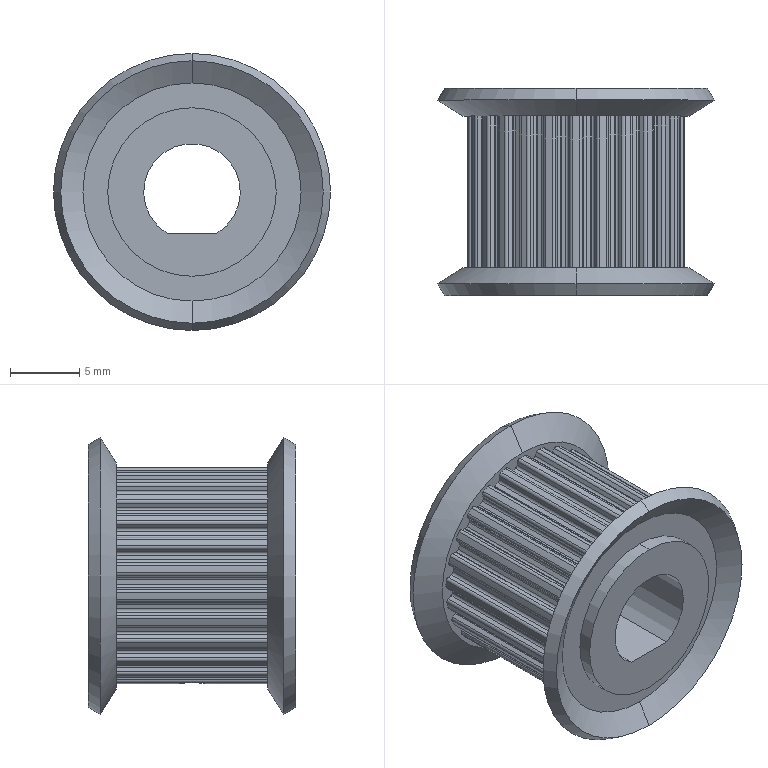Part | NX | features BREP 1 | 1 solid | 257 faces | box 20.061 x 15 x 20.061 mm | volume 2247 mm3 | cylinder 160 | plane 85 | cone 12 | commonest cylinder face diameters 0.46 x126 15.66 x27 12.2 x4 2.5 x2 7 x1